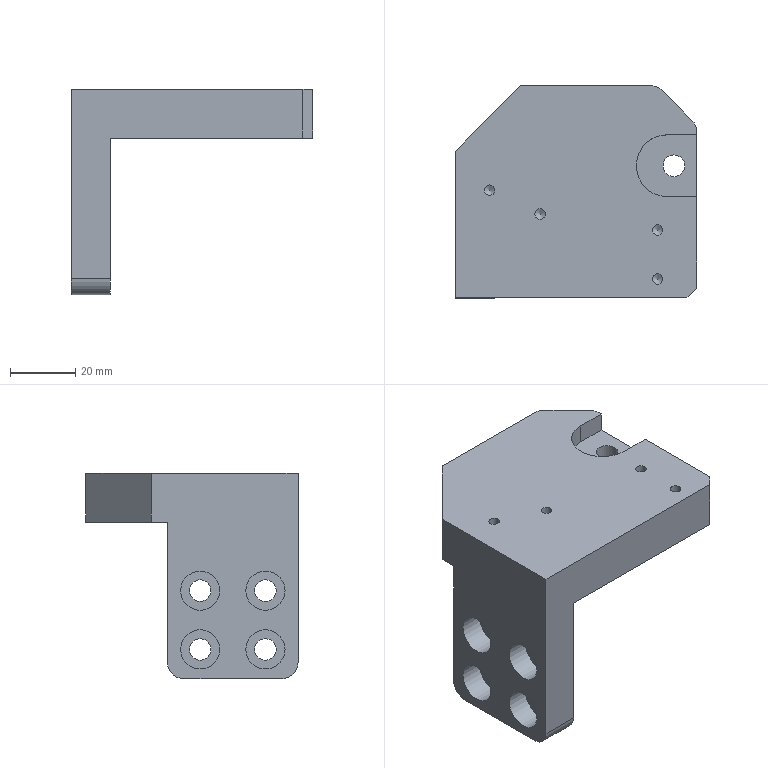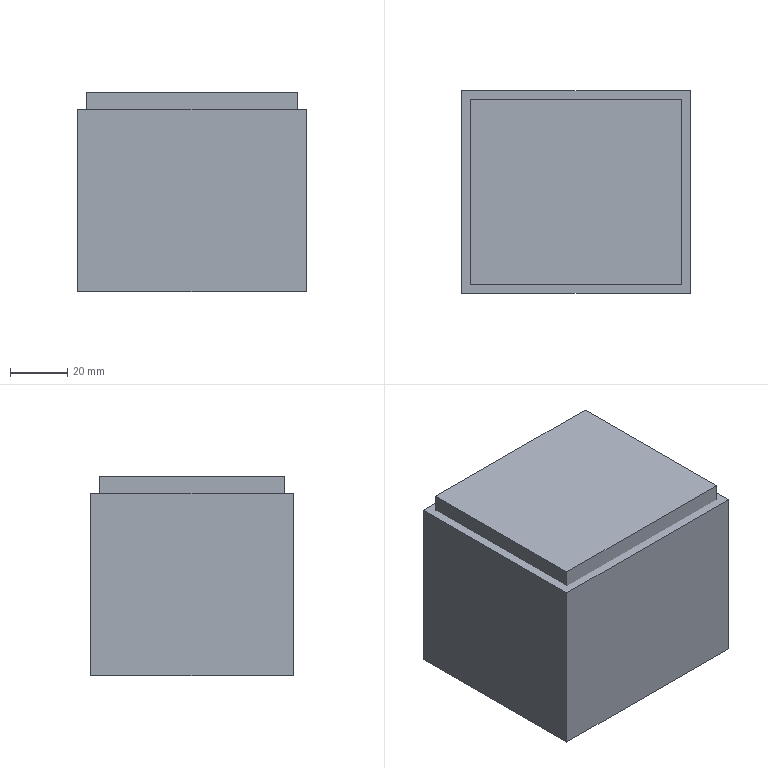CAM job | NX | 3+2 milling, drilling | part box 74 x 65 x 63 mm | stock box 80 x 71 x 70 mm
Tools:
number,name,description,diameter,corner_radius,flute_length,length,flutes
1,D63,Milling Tool-5 Parameters,63.0,0.0,50.0,75.0,2
9,D6A45,Milling Tool-5 Parameters,6.0,0.0,3.0,3.0,2
12,3.2ZT,Drilling Tool,3.2,0.0,35.0,50.0,2
17,D16,Milling Tool-5 Parameters,16.0,0.0,50.0,75.0,2
2,D10,Milling Tool-5 Parameters,10.0,0.0,50.0,75.0,2
18,D6R0.5,Milling Tool-5 Parameters,6.0,0.5,50.0,75.0,2
16,6.6ZT,Drilling Tool,6.6,0.0,35.0,50.0,2
Operations:
program,operation,operation_type,tool,method,geometry_group,spindle_rpm,surface_speed,feed_per_tooth,feed_cut,feed_plunge,cut_length_mm,path_length_mm,cut_time_min,machine_time_min
1-虎钳-80-70-70毛胚,FLOOR_WALL,VolumeBased25DMillingOperation,D63,METHOD,A,6500.0,0.0,0.0,1250.0,100.0,343.797,397.797,0.275,0.2804
1-虎钳-80-70-70毛胚,DRILLING,Operation,D6A45,METHOD,A,4000.0,75.0,0.0312,250.0,0.0,20.0,206.479,0.08,0.0986
1-虎钳-80-70-70毛胚,DRILLING_COPY,Operation,3.2ZT,METHOD,A,2000.0,20.0,0.05,200.0,0.0,55.743,249.633,0.2787,0.2981
1-虎钳-80-70-70毛胚,DRILLING_COPY_COPY,Operation,6.6ZT,METHOD,A,2000.0,20.0,0.05,200.0,0.0,21.483,102.966,0.1074,0.1156
1-虎钳-80-70-70毛胚,ZLEVEL_PROFILE,ZLevelMilling,D16,METHOD,A,6500.0,326.0,0.1538,2000.0,1000.0,19508.525,19628.525,9.778,9.79
1-虎钳-80-70-70毛胚,ZLEVEL_PROFILE_COPY,ZLevelMilling,D16,METHOD,A,6500.0,326.0,0.0769,1000.0,1000.0,1279.73,1466.521,1.28,1.298
1-虎钳-80-70-70毛胚,ZLEVEL_PROFILE_COPY_COPY,ZLevelMilling,D10,METHOD,A,7000.0,219.0,0.1071,1500.0,1000.0,293.05,388.331,0.2011,0.2106
1-虎钳-80-70-70毛胚,ZLEVEL_PROFILE_COPY_1_COPY_COPY_COPY_COPY,ZLevelMilling,D6A45,METHOD,A,7000.0,131.0,0.0714,1000.0,1000.0,318.965,807.912,0.319,0.3679
2-虎钳-80-70-70毛胚,FLOOR_WALL_COPY,VolumeBased25DMillingOperation,D63,METHOD,B,6500.0,0.0,0.0,1250.0,100.0,2280.579,2855.363,1.825,1.882
2-虎钳-80-70-70毛胚,FLOOR_WALL_1,VolumeBased25DMillingOperation,D10,METHOD,B,7000.0,219.0,0.1786,2500.0,1000.0,18404.497,18931.004,7.378,7.431
2-虎钳-80-70-70毛胚,FLOOR_WALL_1_COPY,VolumeBased25DMillingOperation,D10,METHOD,B,7000.0,219.0,0.0714,1000.0,1000.0,238.211,717.661,0.2382,0.2862
2-虎钳-80-70-70毛胚,FLOOR_WALL_1_COPY_COPY,VolumeBased25DMillingOperation,D10,METHOD,B,7000.0,219.0,0.0714,1000.0,1000.0,1166.443,1536.002,1.166,1.203
2-虎钳-80-70-70毛胚,ZLEVEL_PROFILE_1,ZLevelMilling,D6R0.5,METHOD,B,7000.0,131.0,0.1786,2500.0,1000.0,3375.235,3547.605,1.354,1.371
2-虎钳-80-70-70毛胚,ZLEVEL_PROFILE_COPY_1_COPY_COPY_COPY_COPY_COPY,ZLevelMilling,D6A45,METHOD,B,7000.0,131.0,0.0714,1000.0,1000.0,91.919,231.728,0.0919,0.1059
2-虎钳-80-70-70毛胚,ZLEVEL_PROFILE_COPY_1_COPY_COPY_COPY_COPY_COPY_COPY,ZLevelMilling,D6A45,METHOD,B,7000.0,131.0,0.0714,1000.0,1000.0,224.34,607.94,0.2243,0.2627
3-虎钳-80-70-70毛胚,DRILLING_COPY_1,Operation,D6A45,METHOD,C,4000.0,75.0,0.0312,250.0,0.0,16.0,164.571,0.064,0.0789
3-虎钳-80-70-70毛胚,DRILLING_COPY_COPY_COPY,Operation,6.6ZT,METHOD,C,2000.0,20.0,0.05,200.0,0.0,73.931,273.583,0.3697,0.3896
3-虎钳-80-70-70毛胚,HOLE_MILLING,CylinderMilling,D10,METHOD,C,7000.0,219.0,0.1,1400.0,100.0,233.657,556.457,0.1669,0.1992
3-虎钳-80-70-70毛胚,ZLEVEL_PROFILE_COPY_1_COPY_COPY_COPY_COPY_COPY_COPY_COPY,ZLevelMilling,D6A45,METHOD,C,7000.0,131.0,0.0714,1000.0,1000.0,354.076,789.953,0.3541,0.3977